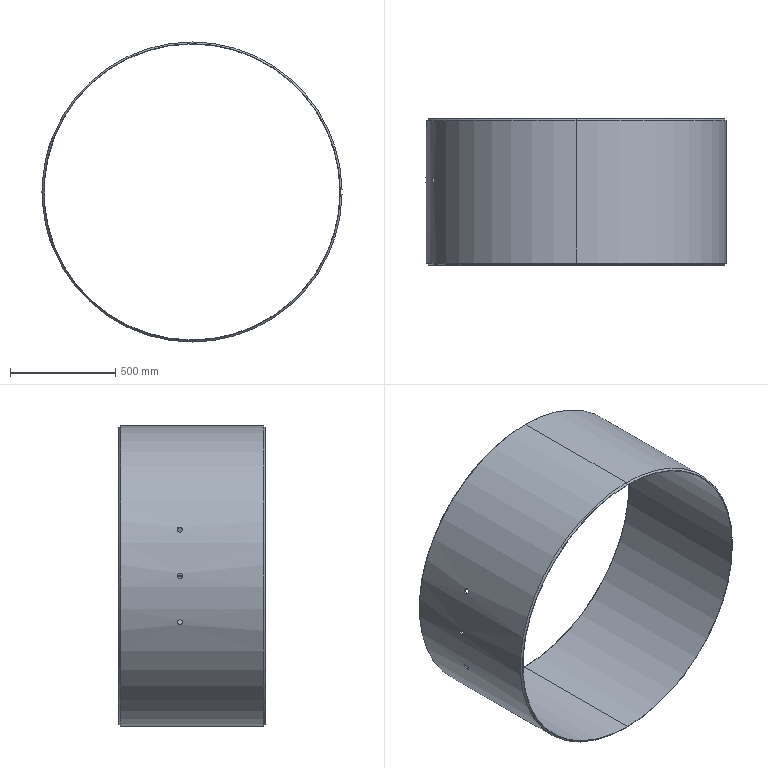Part | SolidWorks | features Chamfer 2, CirPattern 2, FlatPattern 1, HoleWzd 1, SMBaseFlange 1, SheetMetal 1 | 1 solid | 22 faces | box 1428 x 695 x 1428 mm | volume 30589122 mm3 | cylinder 12 | cone 6 | plane 4 | commonest cylinder face diameters 26 x6 1408 x3 1428 x3